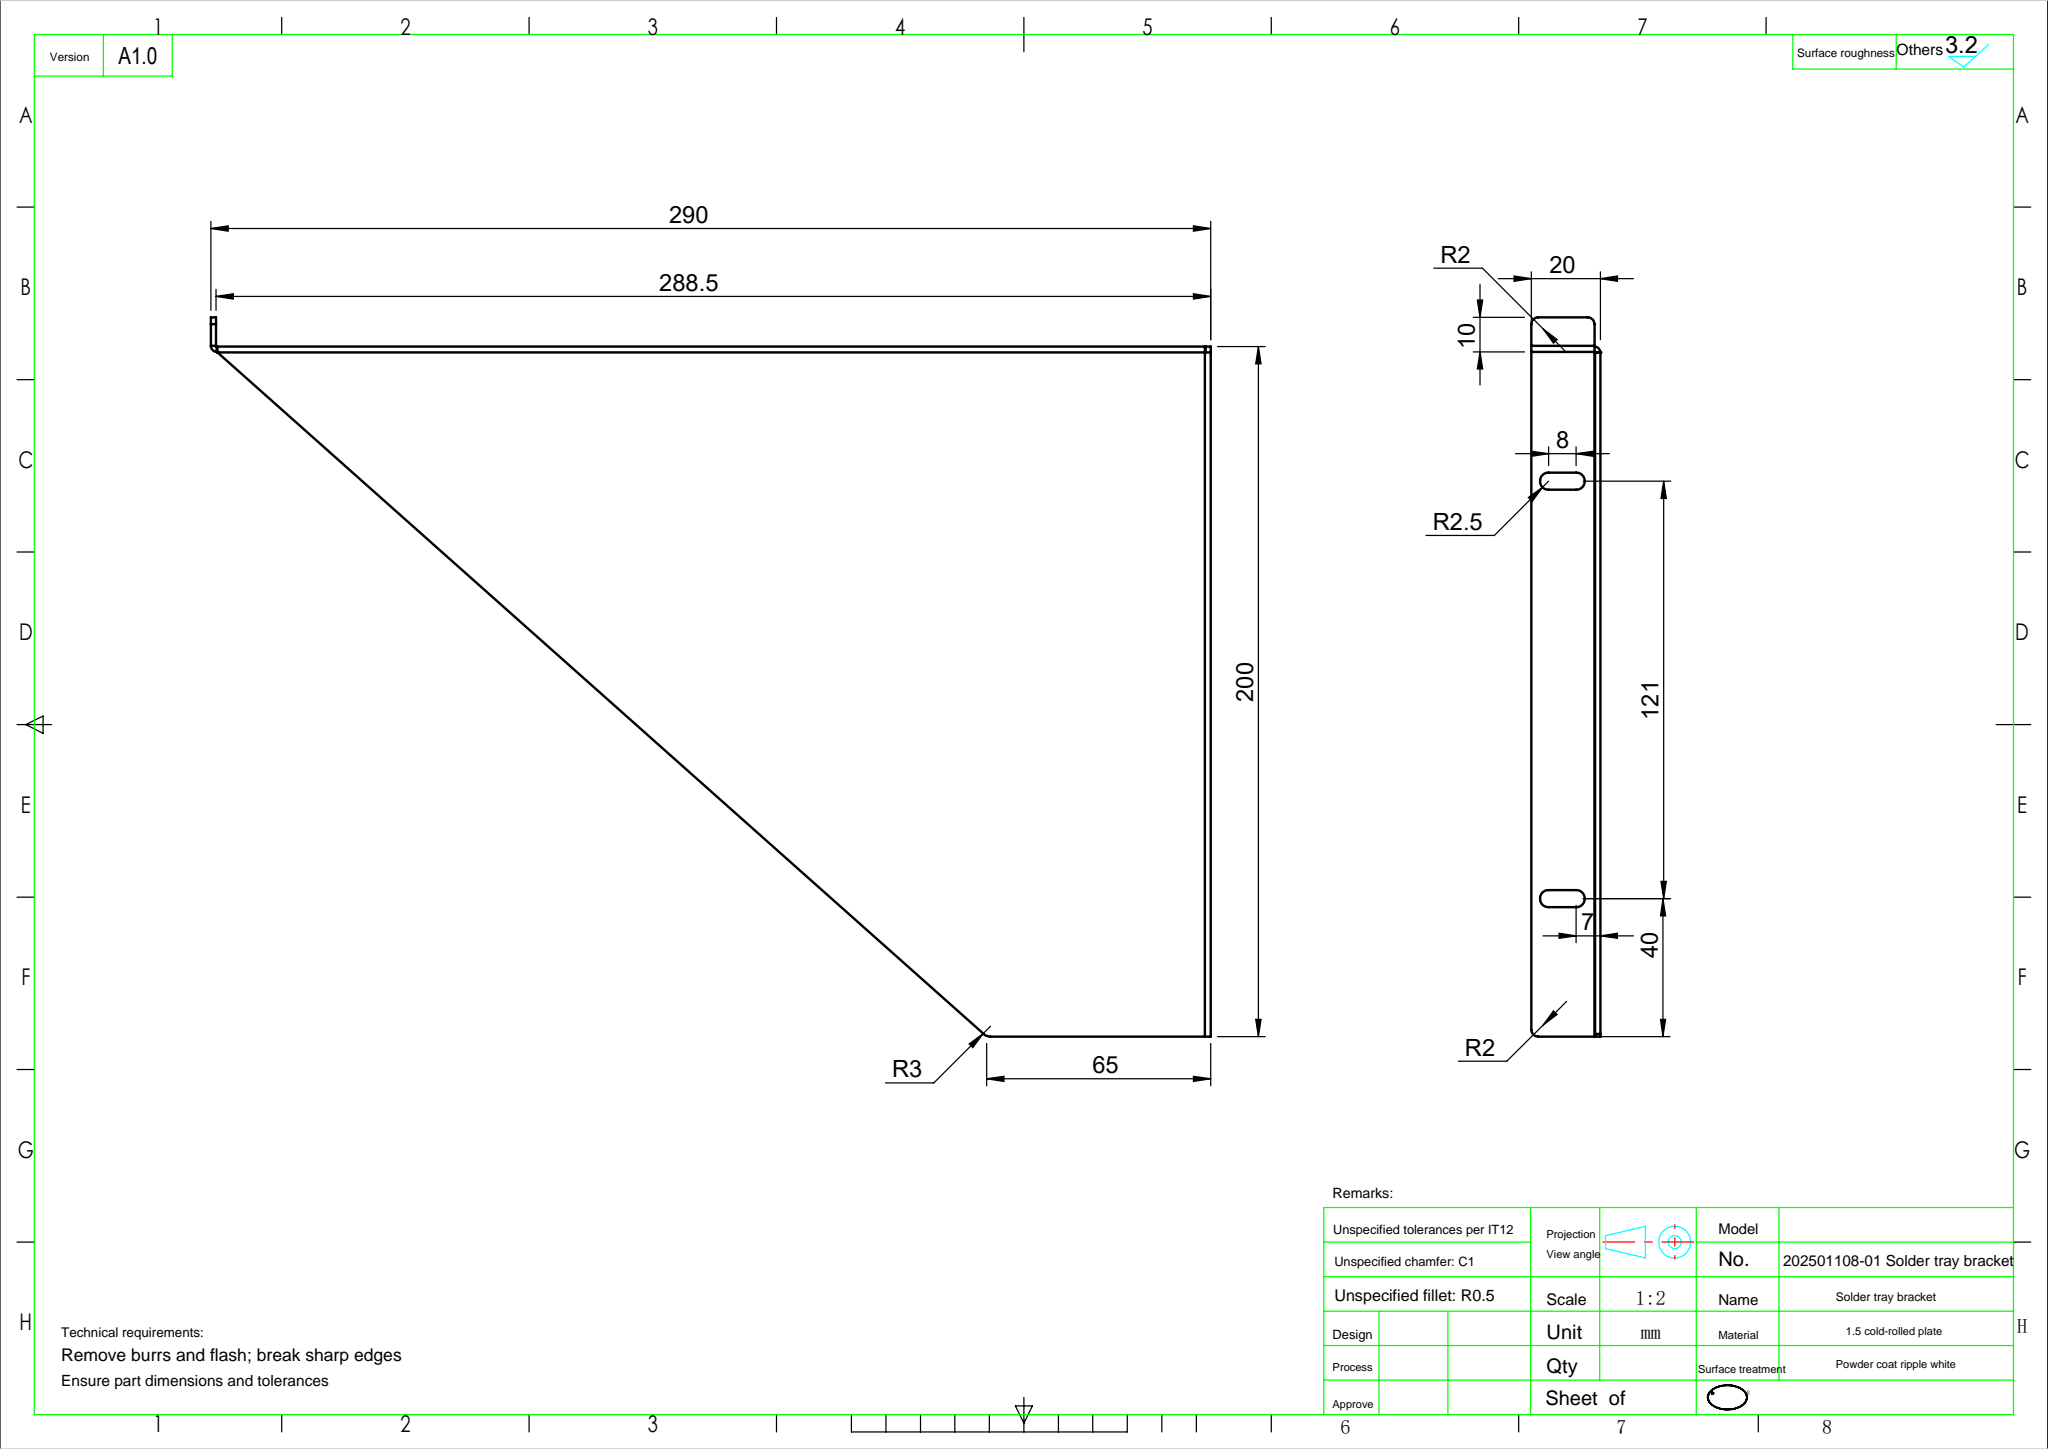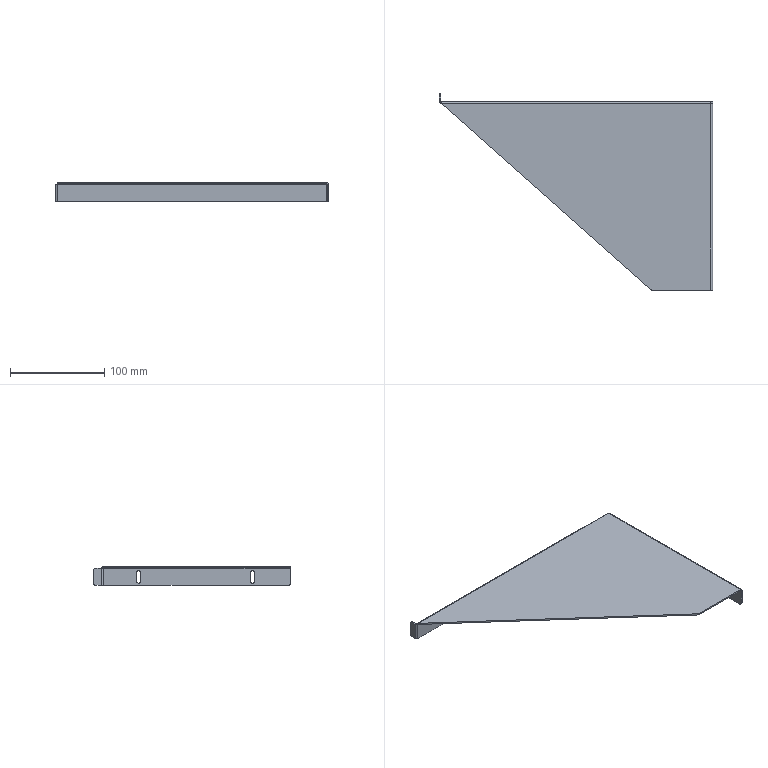Part | SolidWorks | features EdgeFlange 3, Fillet 3, ICE 3, FlatPattern 1, SMBaseFlange 1, SheetMetal 1 | 1 solid | 47 faces | box 290 x 208.5 x 20 mm | volume 66535 mm3 | plane 30 | cylinder 16 | spline 1 | commonest cylinder face diameters 5 x6 0.4 x3 3.4 x3 4 x3 6 x1